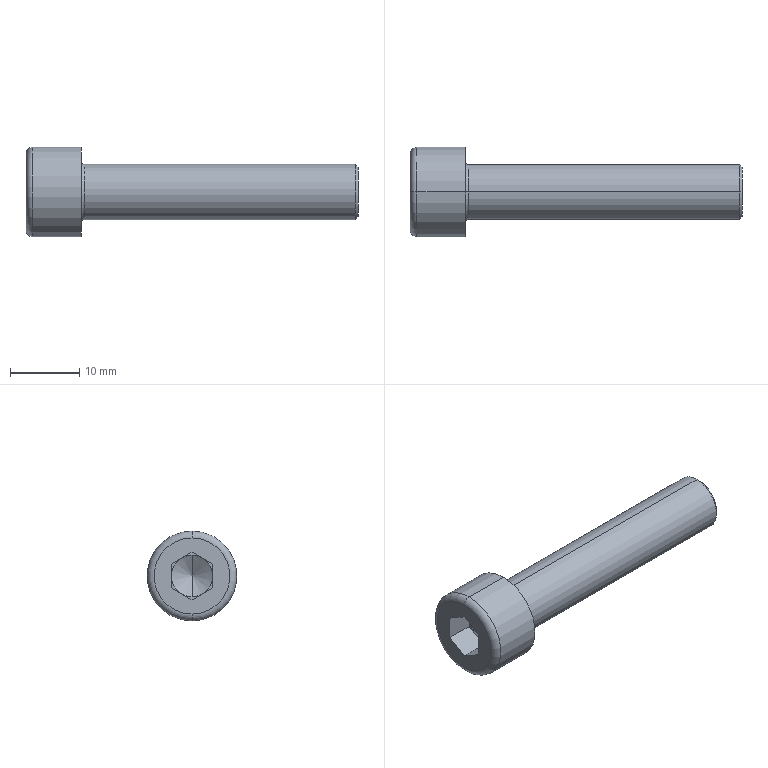Part | NX | features BREP 1 | 1 solid | 27 faces | box 48 x 13 x 13 mm | volume 2922 mm3 | plane 15 | torus 4 | cylinder 4 | cone 4 | commonest cylinder face diameters 8 x2 13 x2
STEP:
#1=CARTESIAN_POINT('',(8.4,0.,4.));
#2=VERTEX_POINT('',#1);
#3=CARTESIAN_POINT('',(8.4,0.,-4.));
#4=VERTEX_POINT('',#3);
#5=CARTESIAN_POINT('',(8.4,0.,0.));
#6=DIRECTION('',(1.,0.,0.));
#7=DIRECTION('',(0.,0.,-1.));
#8=AXIS2_PLACEMENT_3D('',#5,#6,#7);
#9=CIRCLE('',#8,4.);
#10=EDGE_CURVE('',#2,#4,#9,.T.);
#11=ORIENTED_EDGE('',*,*,#10,.F.);
#12=CARTESIAN_POINT('',(8.,0.,4.4));
#13=VERTEX_POINT('',#12);
#14=CARTESIAN_POINT('',(8.4,0.,4.4));
#15=DIRECTION('',(0.,1.,0.));
#16=DIRECTION('',(0.,0.,1.));
#17=AXIS2_PLACEMENT_3D('',#14,#15,#16);
#18=CIRCLE('',#17,0.4);
#19=EDGE_CURVE('',#13,#2,#18,.F.);
#20=ORIENTED_EDGE('',*,*,#19,.F.);
#21=CARTESIAN_POINT('',(8.,0.,-4.4));
#22=VERTEX_POINT('',#21);
#23=CARTESIAN_POINT('',(8.,0.,0.));
#24=DIRECTION('',(-1.,0.,0.));
#25=DIRECTION('',(0.,0.,-1.));
#26=AXIS2_PLACEMENT_3D('',#23,#24,#25);
#27=CIRCLE('',#26,4.4);
#28=EDGE_CURVE('',#22,#13,#27,.T.);
#29=ORIENTED_EDGE('',*,*,#28,.F.);
#30=CARTESIAN_POINT('',(8.4,0.,-4.4));
#31=DIRECTION('',(0.,-1.,0.));
#32=DIRECTION('',(0.,0.,-1.));
#33=AXIS2_PLACEMENT_3D('',#30,#31,#32);
#34=CIRCLE('',#33,0.4);
#35=EDGE_CURVE('',#22,#4,#34,.F.);
#36=ORIENTED_EDGE('',*,*,#35,.T.);
#37=EDGE_LOOP('',(#11,#20,#29,#36));
#38=FACE_BOUND('',#37,.T.);
#39=CARTESIAN_POINT('',(8.4,0.,0.));
#40=DIRECTION('',(1.,0.,0.));
#41=DIRECTION('',(0.,0.,1.));
#42=AXIS2_PLACEMENT_3D('',#39,#40,#41);
#43=TOROIDAL_SURFACE('',#42,4.4,0.4);
#44=ADVANCED_FACE('',(#38),#43,.F.);
#45=CARTESIAN_POINT('',(47.6,0.,-4.));
#46=VERTEX_POINT('',#45);
#47=CARTESIAN_POINT('',(48.,0.,-4.));
#48=DIRECTION('',(-1.,0.,0.));
#49=VECTOR('',#48,1000.);
#50=LINE('',#47,#49);
#51=EDGE_CURVE('',#4,#46,#50,.F.);
#52=ORIENTED_EDGE('',*,*,#51,.T.);
#53=CARTESIAN_POINT('',(47.6,0.,4.));
#54=VERTEX_POINT('',#53);
#55=CARTESIAN_POINT('',(47.6,0.,0.));
#56=DIRECTION('',(-1.,0.,0.));
#57=DIRECTION('',(0.,0.,-1.));
#58=AXIS2_PLACEMENT_3D('',#55,#56,#57);
#59=CIRCLE('',#58,4.);
#60=EDGE_CURVE('',#46,#54,#59,.T.);
#61=ORIENTED_EDGE('',*,*,#60,.T.);
#62=CARTESIAN_POINT('',(48.,0.,4.));
#63=DIRECTION('',(-1.,0.,0.));
#64=VECTOR('',#63,1000.);
#65=LINE('',#62,#64);
#66=EDGE_CURVE('',#2,#54,#65,.F.);
#67=ORIENTED_EDGE('',*,*,#66,.F.);
#68=ORIENTED_EDGE('',*,*,#10,.T.);
#69=EDGE_LOOP('',(#52,#61,#67,#68));
#70=FACE_BOUND('',#69,.T.);
#71=CARTESIAN_POINT('',(48.,0.,0.));
#72=DIRECTION('',(-1.,0.,0.));
#73=DIRECTION('',(0.,0.,-1.));
#74=AXIS2_PLACEMENT_3D('',#71,#72,#73);
#75=CYLINDRICAL_SURFACE('',#74,4.);
#76=ADVANCED_FACE('',(#70),#75,.T.);
#77=ORIENTED_EDGE('',*,*,#28,.T.);
#78=CARTESIAN_POINT('',(8.,0.,0.));
#79=DIRECTION('',(-1.,0.,0.));
#80=DIRECTION('',(0.,0.,-1.));
#81=AXIS2_PLACEMENT_3D('',#78,#79,#80);
#82=CIRCLE('',#81,4.4);
#83=EDGE_CURVE('',#13,#22,#82,.T.);
#84=ORIENTED_EDGE('',*,*,#83,.T.);
#85=EDGE_LOOP('',(#77,#84));
#86=FACE_BOUND('',#85,.T.);
#87=CARTESIAN_POINT('',(8.,0.,6.5));
#88=VERTEX_POINT('',#87);
#89=CARTESIAN_POINT('',(8.,0.,-6.5));
#90=VERTEX_POINT('',#89);
#91=CARTESIAN_POINT('',(8.,0.,0.));
#92=DIRECTION('',(1.,0.,0.));
#93=DIRECTION('',(0.,0.,-1.));
#94=AXIS2_PLACEMENT_3D('',#91,#92,#93);
#95=CIRCLE('',#94,6.5);
#96=EDGE_CURVE('',#88,#90,#95,.T.);
#97=ORIENTED_EDGE('',*,*,#96,.T.);
#98=CARTESIAN_POINT('',(8.,0.,0.));
#99=DIRECTION('',(1.,0.,0.));
#100=DIRECTION('',(0.,0.,-1.));
#101=AXIS2_PLACEMENT_3D('',#98,#99,#100);
#102=CIRCLE('',#101,6.5);
#103=EDGE_CURVE('',#90,#88,#102,.T.);
#104=ORIENTED_EDGE('',*,*,#103,.T.);
#105=EDGE_LOOP('',(#97,#104));
#106=FACE_BOUND('',#105,.T.);
#107=CARTESIAN_POINT('',(8.,0.,0.));
#108=DIRECTION('',(1.,0.,0.));
#109=DIRECTION('',(0.,0.,1.));
#110=AXIS2_PLACEMENT_3D('',#107,#108,#109);
#111=PLANE('',#110);
#112=ADVANCED_FACE('',(#86,#106),#111,.T.);
#113=ORIENTED_EDGE('',*,*,#19,.T.);
#114=CARTESIAN_POINT('',(8.4,0.,0.));
#115=DIRECTION('',(1.,0.,0.));
#116=DIRECTION('',(0.,0.,-1.));
#117=AXIS2_PLACEMENT_3D('',#114,#115,#116);
#118=CIRCLE('',#117,4.);
#119=EDGE_CURVE('',#4,#2,#118,.T.);
#120=ORIENTED_EDGE('',*,*,#119,.F.);
#121=ORIENTED_EDGE('',*,*,#35,.F.);
#122=ORIENTED_EDGE('',*,*,#83,.F.);
#123=EDGE_LOOP('',(#113,#120,#121,#122));
#124=FACE_BOUND('',#123,.T.);
#125=CARTESIAN_POINT('',(8.4,0.,0.));
#126=DIRECTION('',(1.,0.,0.));
#127=DIRECTION('',(0.,0.,1.));
#128=AXIS2_PLACEMENT_3D('',#125,#126,#127);
#129=TOROIDAL_SURFACE('',#128,4.4,0.4);
#130=ADVANCED_FACE('',(#124),#129,.F.);
#131=CARTESIAN_POINT('',(48.,0.,-3.6));
#132=VERTEX_POINT('',#131);
#133=CARTESIAN_POINT('',(48.,0.,-3.6));
#134=DIRECTION('',(-0.7071,0.,-0.7071));
#135=VECTOR('',#134,1000.);
#136=LINE('',#133,#135);
#137=EDGE_CURVE('',#46,#132,#136,.F.);
#138=ORIENTED_EDGE('',*,*,#137,.T.);
#139=CARTESIAN_POINT('',(48.,0.,3.6));
#140=VERTEX_POINT('',#139);
#141=CARTESIAN_POINT('',(48.,0.,0.));
#142=DIRECTION('',(1.,0.,0.));
#143=DIRECTION('',(0.,0.,-1.));
#144=AXIS2_PLACEMENT_3D('',#141,#142,#143);
#145=CIRCLE('',#144,3.6);
#146=EDGE_CURVE('',#140,#132,#145,.T.);
#147=ORIENTED_EDGE('',*,*,#146,.F.);
#148=CARTESIAN_POINT('',(48.,0.,3.6));
#149=DIRECTION('',(-0.7071,0.,0.7071));
#150=VECTOR('',#149,1000.);
#151=LINE('',#148,#150);
#152=EDGE_CURVE('',#54,#140,#151,.F.);
#153=ORIENTED_EDGE('',*,*,#152,.F.);
#154=ORIENTED_EDGE('',*,*,#60,.F.);
#155=EDGE_LOOP('',(#138,#147,#153,#154));
#156=FACE_BOUND('',#155,.T.);
#157=CARTESIAN_POINT('',(48.,0.,0.));
#158=DIRECTION('',(-1.,0.,0.));
#159=DIRECTION('',(0.,0.,-1.));
#160=AXIS2_PLACEMENT_3D('',#157,#158,#159);
#161=CONICAL_SURFACE('',#160,3.6,0.7854);
#162=ADVANCED_FACE('',(#156),#161,.T.);
#163=CARTESIAN_POINT('',(47.6,0.,0.));
#164=DIRECTION('',(-1.,0.,0.));
#165=DIRECTION('',(0.,0.,-1.));
#166=AXIS2_PLACEMENT_3D('',#163,#164,#165);
#167=CIRCLE('',#166,4.);
#168=EDGE_CURVE('',#54,#46,#167,.T.);
#169=ORIENTED_EDGE('',*,*,#168,.T.);
#170=ORIENTED_EDGE('',*,*,#51,.F.);
#171=ORIENTED_EDGE('',*,*,#119,.T.);
#172=ORIENTED_EDGE('',*,*,#66,.T.);
#173=EDGE_LOOP('',(#169,#170,#171,#172));
#174=FACE_BOUND('',#173,.T.);
#175=CARTESIAN_POINT('',(48.,0.,0.));
#176=DIRECTION('',(-1.,0.,0.));
#177=DIRECTION('',(0.,0.,-1.));
#178=AXIS2_PLACEMENT_3D('',#175,#176,#177);
#179=CYLINDRICAL_SURFACE('',#178,4.);
#180=ADVANCED_FACE('',(#174),#179,.T.);
#181=ORIENTED_EDGE('',*,*,#103,.F.);
#182=CARTESIAN_POINT('',(1.,0.,-6.5));
#183=VERTEX_POINT('',#182);
#184=CARTESIAN_POINT('',(8.,0.,-6.5));
#185=DIRECTION('',(-1.,0.,0.));
#186=VECTOR('',#185,1000.);
#187=LINE('',#184,#186);
#188=EDGE_CURVE('',#90,#183,#187,.T.);
#189=ORIENTED_EDGE('',*,*,#188,.T.);
#190=CARTESIAN_POINT('',(1.,0.,6.5));
#191=VERTEX_POINT('',#190);
#192=CARTESIAN_POINT('',(1.,0.,0.));
#193=DIRECTION('',(1.,0.,0.));
#194=DIRECTION('',(0.,0.,-1.));
#195=AXIS2_PLACEMENT_3D('',#192,#193,#194);
#196=CIRCLE('',#195,6.5);
#197=EDGE_CURVE('',#183,#191,#196,.T.);
#198=ORIENTED_EDGE('',*,*,#197,.T.);
#199=CARTESIAN_POINT('',(8.,0.,6.5));
#200=DIRECTION('',(-1.,0.,0.));
#201=VECTOR('',#200,1000.);
#202=LINE('',#199,#201);
#203=EDGE_CURVE('',#88,#191,#202,.T.);
#204=ORIENTED_EDGE('',*,*,#203,.F.);
#205=EDGE_LOOP('',(#181,#189,#198,#204));
#206=FACE_BOUND('',#205,.T.);
#207=CARTESIAN_POINT('',(8.,0.,0.));
#208=DIRECTION('',(-1.,0.,0.));
#209=DIRECTION('',(0.,0.,-1.));
#210=AXIS2_PLACEMENT_3D('',#207,#208,#209);
#211=CYLINDRICAL_SURFACE('',#210,6.5);
#212=ADVANCED_FACE('',(#206),#211,.T.);
#213=ORIENTED_EDGE('',*,*,#188,.F.);
#214=ORIENTED_EDGE('',*,*,#96,.F.);
#215=ORIENTED_EDGE('',*,*,#203,.T.);
#216=CARTESIAN_POINT('',(1.,0.,0.));
#217=DIRECTION('',(1.,0.,0.));
#218=DIRECTION('',(0.,0.,-1.));
#219=AXIS2_PLACEMENT_3D('',#216,#217,#218);
#220=CIRCLE('',#219,6.5);
#221=EDGE_CURVE('',#191,#183,#220,.T.);
#222=ORIENTED_EDGE('',*,*,#221,.T.);
#223=EDGE_LOOP('',(#213,#214,#215,#222));
#224=FACE_BOUND('',#223,.T.);
#225=CARTESIAN_POINT('',(8.,0.,0.));
#226=DIRECTION('',(-1.,0.,0.));
#227=DIRECTION('',(0.,0.,-1.));
#228=AXIS2_PLACEMENT_3D('',#225,#226,#227);
#229=CYLINDRICAL_SURFACE('',#228,6.5);
#230=ADVANCED_FACE('',(#224),#229,.T.);
#231=ORIENTED_EDGE('',*,*,#146,.T.);
#232=CARTESIAN_POINT('',(48.,0.,0.));
#233=DIRECTION('',(1.,0.,0.));
#234=DIRECTION('',(0.,0.,-1.));
#235=AXIS2_PLACEMENT_3D('',#232,#233,#234);
#236=CIRCLE('',#235,3.6);
#237=EDGE_CURVE('',#132,#140,#236,.T.);
#238=ORIENTED_EDGE('',*,*,#237,.T.);
#239=EDGE_LOOP('',(#231,#238));
#240=FACE_BOUND('',#239,.T.);
#241=CARTESIAN_POINT('',(48.,0.,0.));
#242=DIRECTION('',(1.,0.,0.));
#243=DIRECTION('',(0.,0.,1.));
#244=AXIS2_PLACEMENT_3D('',#241,#242,#243);
#245=PLANE('',#244);
#246=ADVANCED_FACE('',(#240),#245,.T.);
#247=ORIENTED_EDGE('',*,*,#237,.F.);
#248=ORIENTED_EDGE('',*,*,#137,.F.);
#249=ORIENTED_EDGE('',*,*,#168,.F.);
#250=ORIENTED_EDGE('',*,*,#152,.T.);
#251=EDGE_LOOP('',(#247,#248,#249,#250));
#252=FACE_BOUND('',#251,.T.);
#253=CARTESIAN_POINT('',(48.,0.,0.));
#254=DIRECTION('',(-1.,0.,0.));
#255=DIRECTION('',(0.,0.,-1.));
#256=AXIS2_PLACEMENT_3D('',#253,#254,#255);
#257=CONICAL_SURFACE('',#256,3.6,0.7854);
#258=ADVANCED_FACE('',(#252),#257,.T.);
#259=CARTESIAN_POINT('',(0.,0.,5.5));
#260=VERTEX_POINT('',#259);
#261=CARTESIAN_POINT('',(0.,0.,-5.5));
#262=VERTEX_POINT('',#261);
#263=CARTESIAN_POINT('',(0.,0.,0.));
#264=DIRECTION('',(-1.,0.,0.));
#265=DIRECTION('',(0.,0.,-1.));
#266=AXIS2_PLACEMENT_3D('',#263,#264,#265);
#267=CIRCLE('',#266,5.5);
#268=EDGE_CURVE('',#260,#262,#267,.T.);
#269=ORIENTED_EDGE('',*,*,#268,.F.);
#270=CARTESIAN_POINT('',(1.,0.,5.5));
#271=DIRECTION('',(0.,1.,0.));
#272=DIRECTION('',(0.,0.,1.));
#273=AXIS2_PLACEMENT_3D('',#270,#271,#272);
#274=CIRCLE('',#273,1.);
#275=EDGE_CURVE('',#191,#260,#274,.F.);
#276=ORIENTED_EDGE('',*,*,#275,.F.);
#277=ORIENTED_EDGE('',*,*,#197,.F.);
#278=CARTESIAN_POINT('',(1.,0.,-5.5));
#279=DIRECTION('',(0.,-1.,0.));
#280=DIRECTION('',(0.,0.,-1.));
#281=AXIS2_PLACEMENT_3D('',#278,#279,#280);
#282=CIRCLE('',#281,1.);
#283=EDGE_CURVE('',#183,#262,#282,.F.);
#284=ORIENTED_EDGE('',*,*,#283,.T.);
#285=EDGE_LOOP('',(#269,#276,#277,#284));
#286=FACE_BOUND('',#285,.T.);
#287=CARTESIAN_POINT('',(1.,0.,0.));
#288=DIRECTION('',(1.,0.,0.));
#289=DIRECTION('',(0.,0.,1.));
#290=AXIS2_PLACEMENT_3D('',#287,#288,#289);
#291=TOROIDAL_SURFACE('',#290,5.5,1.);
#292=ADVANCED_FACE('',(#286),#291,.T.);
#293=ORIENTED_EDGE('',*,*,#275,.T.);
#294=CARTESIAN_POINT('',(0.,0.,0.));
#295=DIRECTION('',(-1.,0.,0.));
#296=DIRECTION('',(0.,0.,-1.));
#297=AXIS2_PLACEMENT_3D('',#294,#295,#296);
#298=CIRCLE('',#297,5.5);
#299=EDGE_CURVE('',#262,#260,#298,.T.);
#300=ORIENTED_EDGE('',*,*,#299,.F.);
#301=ORIENTED_EDGE('',*,*,#283,.F.);
#302=ORIENTED_EDGE('',*,*,#221,.F.);
#303=EDGE_LOOP('',(#293,#300,#301,#302));
#304=FACE_BOUND('',#303,.T.);
#305=CARTESIAN_POINT('',(1.,0.,0.));
#306=DIRECTION('',(1.,0.,0.));
#307=DIRECTION('',(0.,0.,1.));
#308=AXIS2_PLACEMENT_3D('',#305,#306,#307);
#309=TOROIDAL_SURFACE('',#308,5.5,1.);
#310=ADVANCED_FACE('',(#304),#309,.T.);
#311=ORIENTED_EDGE('',*,*,#299,.T.);
#312=ORIENTED_EDGE('',*,*,#268,.T.);
#313=EDGE_LOOP('',(#311,#312));
#314=FACE_BOUND('',#313,.T.);
#315=CARTESIAN_POINT('',(0.,-3.,-1.732));
#316=VERTEX_POINT('',#315);
#317=CARTESIAN_POINT('',(0.,0.,-3.464));
#318=VERTEX_POINT('',#317);
#319=CARTESIAN_POINT('',(0.,-3.,-1.732));
#320=DIRECTION('',(0.,0.866,-0.5));
#321=VECTOR('',#320,1000.);
#322=LINE('',#319,#321);
#323=EDGE_CURVE('',#316,#318,#322,.T.);
#324=ORIENTED_EDGE('',*,*,#323,.T.);
#325=CARTESIAN_POINT('',(0.,3.,-1.732));
#326=VERTEX_POINT('',#325);
#327=CARTESIAN_POINT('',(0.,0.,-3.464));
#328=DIRECTION('',(0.,0.866,0.5));
#329=VECTOR('',#328,1000.);
#330=LINE('',#327,#329);
#331=EDGE_CURVE('',#318,#326,#330,.T.);
#332=ORIENTED_EDGE('',*,*,#331,.T.);
#333=CARTESIAN_POINT('',(0.,3.,1.732));
#334=VERTEX_POINT('',#333);
#335=CARTESIAN_POINT('',(0.,3.,-1.732));
#336=DIRECTION('',(0.,0.,1.));
#337=VECTOR('',#336,1000.);
#338=LINE('',#335,#337);
#339=EDGE_CURVE('',#326,#334,#338,.T.);
#340=ORIENTED_EDGE('',*,*,#339,.T.);
#341=CARTESIAN_POINT('',(0.,0.,3.464));
#342=VERTEX_POINT('',#341);
#343=CARTESIAN_POINT('',(0.,3.,1.732));
#344=DIRECTION('',(0.,-0.866,0.5));
#345=VECTOR('',#344,1000.);
#346=LINE('',#343,#345);
#347=EDGE_CURVE('',#334,#342,#346,.T.);
#348=ORIENTED_EDGE('',*,*,#347,.T.);
#349=CARTESIAN_POINT('',(0.,-3.,1.732));
#350=VERTEX_POINT('',#349);
#351=CARTESIAN_POINT('',(0.,0.,3.464));
#352=DIRECTION('',(0.,-0.866,-0.5));
#353=VECTOR('',#352,1000.);
#354=LINE('',#351,#353);
#355=EDGE_CURVE('',#342,#350,#354,.T.);
#356=ORIENTED_EDGE('',*,*,#355,.T.);
#357=CARTESIAN_POINT('',(0.,-3.,1.732));
#358=DIRECTION('',(0.,0.,-1.));
#359=VECTOR('',#358,1000.);
#360=LINE('',#357,#359);
#361=EDGE_CURVE('',#350,#316,#360,.T.);
#362=ORIENTED_EDGE('',*,*,#361,.T.);
#363=EDGE_LOOP('',(#324,#332,#340,#348,#356,#362));
#364=FACE_BOUND('',#363,.T.);
#365=CARTESIAN_POINT('',(0.,0.,0.));
#366=DIRECTION('',(1.,0.,0.));
#367=DIRECTION('',(0.,0.,1.));
#368=AXIS2_PLACEMENT_3D('',#365,#366,#367);
#369=PLANE('',#368);
#370=ADVANCED_FACE('',(#314,#364),#369,.F.);
#371=ORIENTED_EDGE('',*,*,#361,.F.);
#372=CARTESIAN_POINT('',(4.,-3.,1.732));
#373=VERTEX_POINT('',#372);
#374=CARTESIAN_POINT('',(4.,-3.,1.732));
#375=DIRECTION('',(-1.,0.,0.));
#376=VECTOR('',#375,1000.);
#377=LINE('',#374,#376);
#378=EDGE_CURVE('',#373,#350,#377,.T.);
#379=ORIENTED_EDGE('',*,*,#378,.F.);
#380=CARTESIAN_POINT('',(4.,-3.,0.));
#381=VERTEX_POINT('',#380);
#382=CARTESIAN_POINT('',(4.,-3.,1.732));
#383=DIRECTION('',(0.,0.,-1.));
#384=VECTOR('',#383,1000.);
#385=LINE('',#382,#384);
#386=EDGE_CURVE('',#373,#381,#385,.T.);
#387=ORIENTED_EDGE('',*,*,#386,.T.);
#388=CARTESIAN_POINT('',(4.,-3.,-1.732));
#389=VERTEX_POINT('',#388);
#390=CARTESIAN_POINT('',(4.,-3.,1.732));
#391=DIRECTION('',(0.,0.,-1.));
#392=VECTOR('',#391,1000.);
#393=LINE('',#390,#392);
#394=EDGE_CURVE('',#381,#389,#393,.T.);
#395=ORIENTED_EDGE('',*,*,#394,.T.);
#396=CARTESIAN_POINT('',(4.,-3.,-1.732));
#397=DIRECTION('',(-1.,0.,0.));
#398=VECTOR('',#397,1000.);
#399=LINE('',#396,#398);
#400=EDGE_CURVE('',#389,#316,#399,.T.);
#401=ORIENTED_EDGE('',*,*,#400,.T.);
#402=EDGE_LOOP('',(#371,#379,#387,#395,#401));
#403=FACE_BOUND('',#402,.T.);
#404=CARTESIAN_POINT('',(4.,-3.,1.732));
#405=DIRECTION('',(0.,1.,0.));
#406=DIRECTION('',(0.,0.,-1.));
#407=AXIS2_PLACEMENT_3D('',#404,#405,#406);
#408=PLANE('',#407);
#409=ADVANCED_FACE('',(#403),#408,.T.);
#410=ORIENTED_EDGE('',*,*,#339,.F.);
#411=CARTESIAN_POINT('',(4.,3.,-1.732));
#412=VERTEX_POINT('',#411);
#413=CARTESIAN_POINT('',(4.,3.,-1.732));
#414=DIRECTION('',(-1.,0.,0.));
#415=VECTOR('',#414,1000.);
#416=LINE('',#413,#415);
#417=EDGE_CURVE('',#412,#326,#416,.T.);
#418=ORIENTED_EDGE('',*,*,#417,.F.);
#419=CARTESIAN_POINT('',(4.,3.,0.));
#420=VERTEX_POINT('',#419);
#421=CARTESIAN_POINT('',(4.,3.,-1.732));
#422=DIRECTION('',(0.,0.,1.));
#423=VECTOR('',#422,1000.);
#424=LINE('',#421,#423);
#425=EDGE_CURVE('',#412,#420,#424,.T.);
#426=ORIENTED_EDGE('',*,*,#425,.T.);
#427=CARTESIAN_POINT('',(4.,3.,1.732));
#428=VERTEX_POINT('',#427);
#429=CARTESIAN_POINT('',(4.,3.,-1.732));
#430=DIRECTION('',(0.,0.,1.));
#431=VECTOR('',#430,1000.);
#432=LINE('',#429,#431);
#433=EDGE_CURVE('',#420,#428,#432,.T.);
#434=ORIENTED_EDGE('',*,*,#433,.T.);
#435=CARTESIAN_POINT('',(4.,3.,1.732));
#436=DIRECTION('',(-1.,0.,0.));
#437=VECTOR('',#436,1000.);
#438=LINE('',#435,#437);
#439=EDGE_CURVE('',#428,#334,#438,.T.);
#440=ORIENTED_EDGE('',*,*,#439,.T.);
#441=EDGE_LOOP('',(#410,#418,#426,#434,#440));
#442=FACE_BOUND('',#441,.T.);
#443=CARTESIAN_POINT('',(4.,3.,-1.732));
#444=DIRECTION('',(0.,-1.,0.));
#445=DIRECTION('',(0.,0.,1.));
#446=AXIS2_PLACEMENT_3D('',#443,#444,#445);
#447=PLANE('',#446);
#448=ADVANCED_FACE('',(#442),#447,.T.);
#449=ORIENTED_EDGE('',*,*,#355,.F.);
#450=CARTESIAN_POINT('',(4.,0.,3.464));
#451=VERTEX_POINT('',#450);
#452=CARTESIAN_POINT('',(4.,0.,3.464));
#453=DIRECTION('',(-1.,0.,0.));
#454=VECTOR('',#453,1000.);
#455=LINE('',#452,#454);
#456=EDGE_CURVE('',#451,#342,#455,.T.);
#457=ORIENTED_EDGE('',*,*,#456,.F.);
#458=CARTESIAN_POINT('',(4.,-1.5,2.598));
#459=VERTEX_POINT('',#458);
#460=CARTESIAN_POINT('',(4.,0.,3.464));
#461=DIRECTION('',(0.,-0.866,-0.5));
#462=VECTOR('',#461,1000.);
#463=LINE('',#460,#462);
#464=EDGE_CURVE('',#451,#459,#463,.T.);
#465=ORIENTED_EDGE('',*,*,#464,.T.);
#466=CARTESIAN_POINT('',(4.,0.,3.464));
#467=DIRECTION('',(0.,-0.866,-0.5));
#468=VECTOR('',#467,1000.);
#469=LINE('',#466,#468);
#470=EDGE_CURVE('',#459,#373,#469,.T.);
#471=ORIENTED_EDGE('',*,*,#470,.T.);
#472=ORIENTED_EDGE('',*,*,#378,.T.);
#473=EDGE_LOOP('',(#449,#457,#465,#471,#472));
#474=FACE_BOUND('',#473,.T.);
#475=CARTESIAN_POINT('',(4.,0.,3.464));
#476=DIRECTION('',(0.,0.5,-0.866));
#477=DIRECTION('',(0.,-0.866,-0.5));
#478=AXIS2_PLACEMENT_3D('',#475,#476,#477);
#479=PLANE('',#478);
#480=ADVANCED_FACE('',(#474),#479,.T.);
#481=ORIENTED_EDGE('',*,*,#323,.F.);
#482=ORIENTED_EDGE('',*,*,#400,.F.);
#483=CARTESIAN_POINT('',(4.,-1.5,-2.598));
#484=VERTEX_POINT('',#483);
#485=CARTESIAN_POINT('',(4.,-3.,-1.732));
#486=DIRECTION('',(0.,0.866,-0.5));
#487=VECTOR('',#486,1000.);
#488=LINE('',#485,#487);
#489=EDGE_CURVE('',#389,#484,#488,.T.);
#490=ORIENTED_EDGE('',*,*,#489,.T.);
#491=CARTESIAN_POINT('',(4.,0.,-3.464));
#492=VERTEX_POINT('',#491);
#493=CARTESIAN_POINT('',(4.,-3.,-1.732));
#494=DIRECTION('',(0.,0.866,-0.5));
#495=VECTOR('',#494,1000.);
#496=LINE('',#493,#495);
#497=EDGE_CURVE('',#484,#492,#496,.T.);
#498=ORIENTED_EDGE('',*,*,#497,.T.);
#499=CARTESIAN_POINT('',(4.,0.,-3.464));
#500=DIRECTION('',(-1.,0.,0.));
#501=VECTOR('',#500,1000.);
#502=LINE('',#499,#501);
#503=EDGE_CURVE('',#492,#318,#502,.T.);
#504=ORIENTED_EDGE('',*,*,#503,.T.);
#505=EDGE_LOOP('',(#481,#482,#490,#498,#504));
#506=FACE_BOUND('',#505,.T.);
#507=CARTESIAN_POINT('',(4.,-3.,-1.732));
#508=DIRECTION('',(0.,0.5,0.866));
#509=DIRECTION('',(0.,0.866,-0.5));
#510=AXIS2_PLACEMENT_3D('',#507,#508,#509);
#511=PLANE('',#510);
#512=ADVANCED_FACE('',(#506),#511,.T.);
#513=ORIENTED_EDGE('',*,*,#331,.F.);
#514=ORIENTED_EDGE('',*,*,#503,.F.);
#515=CARTESIAN_POINT('',(4.,1.5,-2.598));
#516=VERTEX_POINT('',#515);
#517=CARTESIAN_POINT('',(4.,0.,-3.464));
#518=DIRECTION('',(0.,0.866,0.5));
#519=VECTOR('',#518,1000.);
#520=LINE('',#517,#519);
#521=EDGE_CURVE('',#492,#516,#520,.T.);
#522=ORIENTED_EDGE('',*,*,#521,.T.);
#523=CARTESIAN_POINT('',(4.,0.,-3.464));
#524=DIRECTION('',(0.,0.866,0.5));
#525=VECTOR('',#524,1000.);
#526=LINE('',#523,#525);
#527=EDGE_CURVE('',#516,#412,#526,.T.);
#528=ORIENTED_EDGE('',*,*,#527,.T.);
#529=ORIENTED_EDGE('',*,*,#417,.T.);
#530=EDGE_LOOP('',(#513,#514,#522,#528,#529));
#531=FACE_BOUND('',#530,.T.);
#532=CARTESIAN_POINT('',(4.,0.,-3.464));
#533=DIRECTION('',(0.,-0.5,0.866));
#534=DIRECTION('',(0.,0.866,0.5));
#535=AXIS2_PLACEMENT_3D('',#532,#533,#534);
#536=PLANE('',#535);
#537=ADVANCED_FACE('',(#531),#536,.T.);
#538=ORIENTED_EDGE('',*,*,#347,.F.);
#539=ORIENTED_EDGE('',*,*,#439,.F.);
#540=CARTESIAN_POINT('',(4.,1.5,2.598));
#541=VERTEX_POINT('',#540);
#542=CARTESIAN_POINT('',(4.,3.,1.732));
#543=DIRECTION('',(0.,-0.866,0.5));
#544=VECTOR('',#543,1000.);
#545=LINE('',#542,#544);
#546=EDGE_CURVE('',#428,#541,#545,.T.);
#547=ORIENTED_EDGE('',*,*,#546,.T.);
#548=CARTESIAN_POINT('',(4.,3.,1.732));
#549=DIRECTION('',(0.,-0.866,0.5));
#550=VECTOR('',#549,1000.);
#551=LINE('',#548,#550);
#552=EDGE_CURVE('',#541,#451,#551,.T.);
#553=ORIENTED_EDGE('',*,*,#552,.T.);
#554=ORIENTED_EDGE('',*,*,#456,.T.);
#555=EDGE_LOOP('',(#538,#539,#547,#553,#554));
#556=FACE_BOUND('',#555,.T.);
#557=CARTESIAN_POINT('',(4.,3.,1.732));
#558=DIRECTION('',(0.,-0.5,-0.866));
#559=DIRECTION('',(0.,-0.866,0.5));
#560=AXIS2_PLACEMENT_3D('',#557,#558,#559);
#561=PLANE('',#560);
#562=ADVANCED_FACE('',(#556),#561,.T.);
#563=ORIENTED_EDGE('',*,*,#394,.F.);
#564=CARTESIAN_POINT('',(4.,0.,0.));
#565=DIRECTION('',(1.,0.,0.));
#566=DIRECTION('',(0.,0.,-1.));
#567=AXIS2_PLACEMENT_3D('',#564,#565,#566);
#568=CIRCLE('',#567,3.);
#569=EDGE_CURVE('',#381,#484,#568,.T.);
#570=ORIENTED_EDGE('',*,*,#569,.T.);
#571=ORIENTED_EDGE('',*,*,#489,.F.);
#572=EDGE_LOOP('',(#563,#570,#571));
#573=FACE_BOUND('',#572,.T.);
#574=CARTESIAN_POINT('',(4.,0.,-3.464));
#575=DIRECTION('',(1.,0.,0.));
#576=DIRECTION('',(0.,0.,1.));
#577=AXIS2_PLACEMENT_3D('',#574,#575,#576);
#578=PLANE('',#577);
#579=ADVANCED_FACE('',(#573),#578,.F.);
#580=ORIENTED_EDGE('',*,*,#470,.F.);
#581=CARTESIAN_POINT('',(4.,0.,0.));
#582=DIRECTION('',(1.,0.,0.));
#583=DIRECTION('',(0.,0.,-1.));
#584=AXIS2_PLACEMENT_3D('',#581,#582,#583);
#585=CIRCLE('',#584,3.);
#586=EDGE_CURVE('',#459,#381,#585,.T.);
#587=ORIENTED_EDGE('',*,*,#586,.T.);
#588=ORIENTED_EDGE('',*,*,#386,.F.);
#589=EDGE_LOOP('',(#580,#587,#588));
#590=FACE_BOUND('',#589,.T.);
#591=CARTESIAN_POINT('',(4.,0.,-3.464));
#592=DIRECTION('',(1.,0.,0.));
#593=DIRECTION('',(0.,0.,1.));
#594=AXIS2_PLACEMENT_3D('',#591,#592,#593);
#595=PLANE('',#594);
#596=ADVANCED_FACE('',(#590),#595,.F.);
#597=ORIENTED_EDGE('',*,*,#527,.F.);
#598=CARTESIAN_POINT('',(4.,0.,0.));
#599=DIRECTION('',(1.,0.,0.));
#600=DIRECTION('',(0.,0.,-1.));
#601=AXIS2_PLACEMENT_3D('',#598,#599,#600);
#602=CIRCLE('',#601,3.);
#603=EDGE_CURVE('',#516,#420,#602,.T.);
#604=ORIENTED_EDGE('',*,*,#603,.T.);
#605=ORIENTED_EDGE('',*,*,#425,.F.);
#606=EDGE_LOOP('',(#597,#604,#605));
#607=FACE_BOUND('',#606,.T.);
#608=CARTESIAN_POINT('',(4.,0.,-3.464));
#609=DIRECTION('',(1.,0.,0.));
#610=DIRECTION('',(0.,0.,1.));
#611=AXIS2_PLACEMENT_3D('',#608,#609,#610);
#612=PLANE('',#611);
#613=ADVANCED_FACE('',(#607),#612,.F.);
#614=ORIENTED_EDGE('',*,*,#433,.F.);
#615=CARTESIAN_POINT('',(4.,0.,0.));
#616=DIRECTION('',(1.,0.,0.));
#617=DIRECTION('',(0.,0.,-1.));
#618=AXIS2_PLACEMENT_3D('',#615,#616,#617);
#619=CIRCLE('',#618,3.);
#620=EDGE_CURVE('',#420,#541,#619,.T.);
#621=ORIENTED_EDGE('',*,*,#620,.T.);
#622=ORIENTED_EDGE('',*,*,#546,.F.);
#623=EDGE_LOOP('',(#614,#621,#622));
#624=FACE_BOUND('',#623,.T.);
#625=CARTESIAN_POINT('',(4.,0.,-3.464));
#626=DIRECTION('',(1.,0.,0.));
#627=DIRECTION('',(0.,0.,1.));
#628=AXIS2_PLACEMENT_3D('',#625,#626,#627);
#629=PLANE('',#628);
#630=ADVANCED_FACE('',(#624),#629,.F.);
#631=ORIENTED_EDGE('',*,*,#552,.F.);
#632=CARTESIAN_POINT('',(4.,0.,3.));
#633=VERTEX_POINT('',#632);
#634=CARTESIAN_POINT('',(4.,0.,0.));
#635=DIRECTION('',(1.,0.,0.));
#636=DIRECTION('',(0.,0.,-1.));
#637=AXIS2_PLACEMENT_3D('',#634,#635,#636);
#638=CIRCLE('',#637,3.);
#639=EDGE_CURVE('',#541,#633,#638,.T.);
#640=ORIENTED_EDGE('',*,*,#639,.T.);
#641=CARTESIAN_POINT('',(4.,0.,0.));
#642=DIRECTION('',(1.,0.,0.));
#643=DIRECTION('',(0.,0.,-1.));
#644=AXIS2_PLACEMENT_3D('',#641,#642,#643);
#645=CIRCLE('',#644,3.);
#646=EDGE_CURVE('',#633,#459,#645,.T.);
#647=ORIENTED_EDGE('',*,*,#646,.T.);
#648=ORIENTED_EDGE('',*,*,#464,.F.);
#649=EDGE_LOOP('',(#631,#640,#647,#648));
#650=FACE_BOUND('',#649,.T.);
#651=CARTESIAN_POINT('',(4.,0.,-3.464));
#652=DIRECTION('',(1.,0.,0.));
#653=DIRECTION('',(0.,0.,1.));
#654=AXIS2_PLACEMENT_3D('',#651,#652,#653);
#655=PLANE('',#654);
#656=ADVANCED_FACE('',(#650),#655,.F.);
#657=ORIENTED_EDGE('',*,*,#497,.F.);
#658=CARTESIAN_POINT('',(4.,0.,-3.));
#659=VERTEX_POINT('',#658);
#660=CARTESIAN_POINT('',(4.,0.,0.));
#661=DIRECTION('',(1.,0.,0.));
#662=DIRECTION('',(0.,0.,-1.));
#663=AXIS2_PLACEMENT_3D('',#660,#661,#662);
#664=CIRCLE('',#663,3.);
#665=EDGE_CURVE('',#484,#659,#664,.T.);
#666=ORIENTED_EDGE('',*,*,#665,.T.);
#667=CARTESIAN_POINT('',(4.,0.,0.));
#668=DIRECTION('',(1.,0.,0.));
#669=DIRECTION('',(0.,0.,-1.));
#670=AXIS2_PLACEMENT_3D('',#667,#668,#669);
#671=CIRCLE('',#670,3.);
#672=EDGE_CURVE('',#659,#516,#671,.T.);
#673=ORIENTED_EDGE('',*,*,#672,.T.);
#674=ORIENTED_EDGE('',*,*,#521,.F.);
#675=EDGE_LOOP('',(#657,#666,#673,#674));
#676=FACE_BOUND('',#675,.T.);
#677=CARTESIAN_POINT('',(4.,0.,-3.464));
#678=DIRECTION('',(1.,0.,0.));
#679=DIRECTION('',(0.,0.,1.));
#680=AXIS2_PLACEMENT_3D('',#677,#678,#679);
#681=PLANE('',#680);
#682=ADVANCED_FACE('',(#676),#681,.F.);
#683=CARTESIAN_POINT('',(5.732,0.,0.));
#684=VERTEX_POINT('',#683);
#685=CARTESIAN_POINT('',(4.,0.,3.));
#686=DIRECTION('',(-0.5,0.,0.866));
#687=VECTOR('',#686,1000.);
#688=LINE('',#685,#687);
#689=EDGE_CURVE('',#684,#633,#688,.T.);
#690=ORIENTED_EDGE('',*,*,#689,.F.);
#691=CARTESIAN_POINT('',(4.,0.,-3.));
#692=DIRECTION('',(-0.5,0.,-0.866));
#693=VECTOR('',#692,1000.);
#694=LINE('',#691,#693);
#695=EDGE_CURVE('',#684,#659,#694,.T.);
#696=ORIENTED_EDGE('',*,*,#695,.T.);
#697=ORIENTED_EDGE('',*,*,#665,.F.);
#698=ORIENTED_EDGE('',*,*,#569,.F.);
#699=ORIENTED_EDGE('',*,*,#586,.F.);
#700=ORIENTED_EDGE('',*,*,#646,.F.);
#701=EDGE_LOOP('',(#690,#696,#697,#698,#699,#700));
#702=FACE_BOUND('',#701,.T.);
#703=CARTESIAN_POINT('',(4.,0.,0.));
#704=DIRECTION('',(-1.,0.,0.));
#705=DIRECTION('',(0.,0.,-1.));
#706=AXIS2_PLACEMENT_3D('',#703,#704,#705);
#707=CONICAL_SURFACE('',#706,3.,1.047);
#708=ADVANCED_FACE('',(#702),#707,.F.);
#709=ORIENTED_EDGE('',*,*,#695,.F.);
#710=ORIENTED_EDGE('',*,*,#689,.T.);
#711=ORIENTED_EDGE('',*,*,#639,.F.);
#712=ORIENTED_EDGE('',*,*,#620,.F.);
#713=ORIENTED_EDGE('',*,*,#603,.F.);
#714=ORIENTED_EDGE('',*,*,#672,.F.);
#715=EDGE_LOOP('',(#709,#710,#711,#712,#713,#714));
#716=FACE_BOUND('',#715,.T.);
#717=CARTESIAN_POINT('',(4.,0.,0.));
#718=DIRECTION('',(-1.,0.,0.));
#719=DIRECTION('',(0.,0.,-1.));
#720=AXIS2_PLACEMENT_3D('',#717,#718,#719);
#721=CONICAL_SURFACE('',#720,3.,1.047);
#722=ADVANCED_FACE('',(#716),#721,.F.);
#723=CLOSED_SHELL('',(#44,#76,#112,#130,#162,#180,#212,#230,#246,#258,#292,#310,#370,#409,#448,#480,#512,#537,#562,#579,#596,#613,#630,#656,#682,#708,#722));
#724=MANIFOLD_SOLID_BREP('',#723);
#725=(LENGTH_UNIT()NAMED_UNIT(*)SI_UNIT(.MILLI.,.METRE.));
#726=UNCERTAINTY_MEASURE_WITH_UNIT(LENGTH_MEASURE(0.00001),#725,'','');
#727=(NAMED_UNIT(*)PLANE_ANGLE_UNIT()SI_UNIT($,.RADIAN.));
#728=(NAMED_UNIT(*)SI_UNIT($,.STERADIAN.)SOLID_ANGLE_UNIT());
#729=(GEOMETRIC_REPRESENTATION_CONTEXT(3)GLOBAL_UNCERTAINTY_ASSIGNED_CONTEXT((#726))GLOBAL_UNIT_ASSIGNED_CONTEXT((#725,#727,#728))REPRESENTATION_CONTEXT('',''));
#730=ADVANCED_BREP_SHAPE_REPRESENTATION('',(#724),#729);